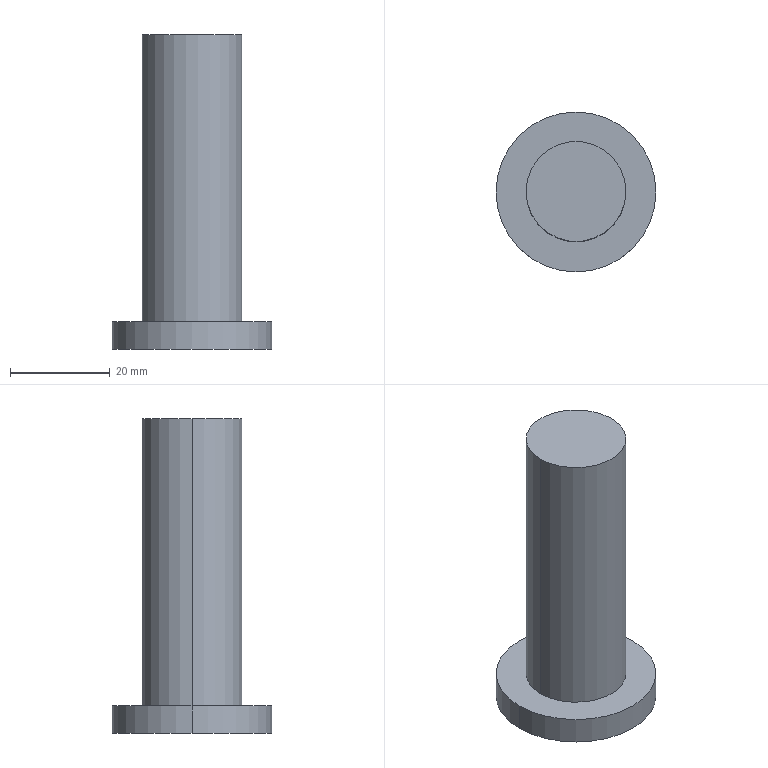Part | SolidWorks | features Extrusion 1, ICE 1 | 1 solid | 7 faces | box 32 x 32 x 63 mm | volume 22488 mm3 | cylinder 4 | plane 3 | commonest cylinder face diameters 20 x2 32 x2
STEP:
#1=CARTESIAN_POINT('',(16.,0.,5.5));
#2=VERTEX_POINT('',#1);
#3=CARTESIAN_POINT('',(-16.,0.,5.5));
#4=VERTEX_POINT('',#3);
#5=CARTESIAN_POINT('',(0.,0.,5.5));
#6=DIRECTION('',(0.,0.,1.));
#7=DIRECTION('',(1.,0.,0.));
#8=AXIS2_PLACEMENT_3D('',#5,#6,#7);
#9=CIRCLE('',#8,16.);
#10=EDGE_CURVE('',#2,#4,#9,.T.);
#11=ORIENTED_EDGE('',*,*,#10,.F.);
#12=CARTESIAN_POINT('',(16.,0.,0.));
#13=VERTEX_POINT('',#12);
#14=CARTESIAN_POINT('',(16.,0.,5.5));
#15=DIRECTION('',(0.,0.,-1.));
#16=VECTOR('',#15,1000.);
#17=LINE('',#14,#16);
#18=EDGE_CURVE('',#2,#13,#17,.T.);
#19=ORIENTED_EDGE('',*,*,#18,.T.);
#20=CARTESIAN_POINT('',(-16.,0.,0.));
#21=VERTEX_POINT('',#20);
#22=CARTESIAN_POINT('',(0.,0.,0.));
#23=DIRECTION('',(0.,0.,1.));
#24=DIRECTION('',(1.,0.,0.));
#25=AXIS2_PLACEMENT_3D('',#22,#23,#24);
#26=CIRCLE('',#25,16.);
#27=EDGE_CURVE('',#13,#21,#26,.T.);
#28=ORIENTED_EDGE('',*,*,#27,.T.);
#29=CARTESIAN_POINT('',(-16.,0.,5.5));
#30=DIRECTION('',(0.,0.,-1.));
#31=VECTOR('',#30,1000.);
#32=LINE('',#29,#31);
#33=EDGE_CURVE('',#4,#21,#32,.T.);
#34=ORIENTED_EDGE('',*,*,#33,.F.);
#35=EDGE_LOOP('',(#11,#19,#28,#34));
#36=FACE_OUTER_BOUND('',#35,.T.);
#37=CARTESIAN_POINT('',(0.,0.,5.5));
#38=DIRECTION('',(0.,0.,-1.));
#39=DIRECTION('',(-1.,0.,0.));
#40=AXIS2_PLACEMENT_3D('',#37,#38,#39);
#41=CYLINDRICAL_SURFACE('',#40,16.);
#42=ADVANCED_FACE('',(#36),#41,.T.);
#43=CARTESIAN_POINT('',(10.,0.,63.));
#44=VERTEX_POINT('',#43);
#45=CARTESIAN_POINT('',(-10.,0.,63.));
#46=VERTEX_POINT('',#45);
#47=CARTESIAN_POINT('',(0.,0.,63.));
#48=DIRECTION('',(0.,0.,1.));
#49=DIRECTION('',(1.,0.,0.));
#50=AXIS2_PLACEMENT_3D('',#47,#48,#49);
#51=CIRCLE('',#50,10.);
#52=EDGE_CURVE('',#44,#46,#51,.T.);
#53=ORIENTED_EDGE('',*,*,#52,.F.);
#54=CARTESIAN_POINT('',(10.,0.,5.5));
#55=VERTEX_POINT('',#54);
#56=CARTESIAN_POINT('',(10.,0.,63.));
#57=DIRECTION('',(0.,0.,-1.));
#58=VECTOR('',#57,1000.);
#59=LINE('',#56,#58);
#60=EDGE_CURVE('',#44,#55,#59,.T.);
#61=ORIENTED_EDGE('',*,*,#60,.T.);
#62=CARTESIAN_POINT('',(-10.,0.,5.5));
#63=VERTEX_POINT('',#62);
#64=CARTESIAN_POINT('',(0.,0.,5.5));
#65=DIRECTION('',(0.,0.,1.));
#66=DIRECTION('',(1.,0.,0.));
#67=AXIS2_PLACEMENT_3D('',#64,#65,#66);
#68=CIRCLE('',#67,10.);
#69=EDGE_CURVE('',#55,#63,#68,.T.);
#70=ORIENTED_EDGE('',*,*,#69,.T.);
#71=CARTESIAN_POINT('',(-10.,0.,63.));
#72=DIRECTION('',(0.,0.,-1.));
#73=VECTOR('',#72,1000.);
#74=LINE('',#71,#73);
#75=EDGE_CURVE('',#46,#63,#74,.T.);
#76=ORIENTED_EDGE('',*,*,#75,.F.);
#77=EDGE_LOOP('',(#53,#61,#70,#76));
#78=FACE_OUTER_BOUND('',#77,.T.);
#79=CARTESIAN_POINT('',(0.,0.,63.));
#80=DIRECTION('',(0.,0.,-1.));
#81=DIRECTION('',(-1.,0.,0.));
#82=AXIS2_PLACEMENT_3D('',#79,#80,#81);
#83=CYLINDRICAL_SURFACE('',#82,10.);
#84=ADVANCED_FACE('',(#78),#83,.T.);
#85=ORIENTED_EDGE('',*,*,#60,.F.);
#86=CARTESIAN_POINT('',(0.,0.,63.));
#87=DIRECTION('',(0.,0.,1.));
#88=DIRECTION('',(1.,0.,0.));
#89=AXIS2_PLACEMENT_3D('',#86,#87,#88);
#90=CIRCLE('',#89,10.);
#91=EDGE_CURVE('',#46,#44,#90,.T.);
#92=ORIENTED_EDGE('',*,*,#91,.F.);
#93=ORIENTED_EDGE('',*,*,#75,.T.);
#94=CARTESIAN_POINT('',(0.,0.,5.5));
#95=DIRECTION('',(0.,0.,1.));
#96=DIRECTION('',(1.,0.,0.));
#97=AXIS2_PLACEMENT_3D('',#94,#95,#96);
#98=CIRCLE('',#97,10.);
#99=EDGE_CURVE('',#63,#55,#98,.T.);
#100=ORIENTED_EDGE('',*,*,#99,.T.);
#101=EDGE_LOOP('',(#85,#92,#93,#100));
#102=FACE_OUTER_BOUND('',#101,.T.);
#103=CARTESIAN_POINT('',(0.,0.,63.));
#104=DIRECTION('',(0.,0.,-1.));
#105=DIRECTION('',(-1.,0.,0.));
#106=AXIS2_PLACEMENT_3D('',#103,#104,#105);
#107=CYLINDRICAL_SURFACE('',#106,10.);
#108=ADVANCED_FACE('',(#102),#107,.T.);
#109=ORIENTED_EDGE('',*,*,#91,.T.);
#110=ORIENTED_EDGE('',*,*,#52,.T.);
#111=EDGE_LOOP('',(#109,#110));
#112=FACE_OUTER_BOUND('',#111,.T.);
#113=CARTESIAN_POINT('',(0.,0.,63.));
#114=DIRECTION('',(0.,0.,1.));
#115=DIRECTION('',(1.,0.,0.));
#116=AXIS2_PLACEMENT_3D('',#113,#114,#115);
#117=PLANE('',#116);
#118=ADVANCED_FACE('',(#112),#117,.T.);
#119=ORIENTED_EDGE('',*,*,#18,.F.);
#120=CARTESIAN_POINT('',(0.,0.,5.5));
#121=DIRECTION('',(0.,0.,1.));
#122=DIRECTION('',(1.,0.,0.));
#123=AXIS2_PLACEMENT_3D('',#120,#121,#122);
#124=CIRCLE('',#123,16.);
#125=EDGE_CURVE('',#4,#2,#124,.T.);
#126=ORIENTED_EDGE('',*,*,#125,.F.);
#127=ORIENTED_EDGE('',*,*,#33,.T.);
#128=CARTESIAN_POINT('',(0.,0.,0.));
#129=DIRECTION('',(0.,0.,1.));
#130=DIRECTION('',(1.,0.,0.));
#131=AXIS2_PLACEMENT_3D('',#128,#129,#130);
#132=CIRCLE('',#131,16.);
#133=EDGE_CURVE('',#21,#13,#132,.T.);
#134=ORIENTED_EDGE('',*,*,#133,.T.);
#135=EDGE_LOOP('',(#119,#126,#127,#134));
#136=FACE_OUTER_BOUND('',#135,.T.);
#137=CARTESIAN_POINT('',(0.,0.,5.5));
#138=DIRECTION('',(0.,0.,-1.));
#139=DIRECTION('',(-1.,0.,0.));
#140=AXIS2_PLACEMENT_3D('',#137,#138,#139);
#141=CYLINDRICAL_SURFACE('',#140,16.);
#142=ADVANCED_FACE('',(#136),#141,.T.);
#143=ORIENTED_EDGE('',*,*,#99,.F.);
#144=ORIENTED_EDGE('',*,*,#69,.F.);
#145=EDGE_LOOP('',(#143,#144));
#146=FACE_BOUND('',#145,.T.);
#147=ORIENTED_EDGE('',*,*,#125,.T.);
#148=ORIENTED_EDGE('',*,*,#10,.T.);
#149=EDGE_LOOP('',(#147,#148));
#150=FACE_OUTER_BOUND('',#149,.T.);
#151=CARTESIAN_POINT('',(0.,0.,5.5));
#152=DIRECTION('',(0.,0.,1.));
#153=DIRECTION('',(1.,0.,0.));
#154=AXIS2_PLACEMENT_3D('',#151,#152,#153);
#155=PLANE('',#154);
#156=ADVANCED_FACE('',(#146,#150),#155,.T.);
#157=ORIENTED_EDGE('',*,*,#133,.F.);
#158=ORIENTED_EDGE('',*,*,#27,.F.);
#159=EDGE_LOOP('',(#157,#158));
#160=FACE_OUTER_BOUND('',#159,.T.);
#161=CARTESIAN_POINT('',(0.,0.,0.));
#162=DIRECTION('',(0.,0.,1.));
#163=DIRECTION('',(1.,0.,0.));
#164=AXIS2_PLACEMENT_3D('',#161,#162,#163);
#165=PLANE('',#164);
#166=ADVANCED_FACE('',(#160),#165,.F.);
#167=CLOSED_SHELL('',(#42,#84,#108,#118,#142,#156,#166));
#168=MANIFOLD_SOLID_BREP('',#167);
#169=CARTESIAN_POINT('',(0.,0.,0.));
#170=DIRECTION('',(0.,0.,1.));
#171=DIRECTION('',(1.,0.,0.));
#172=AXIS2_PLACEMENT_3D('',#169,#170,#171);
#173=(LENGTH_UNIT()NAMED_UNIT(*)SI_UNIT(.MILLI.,.METRE.));
#174=UNCERTAINTY_MEASURE_WITH_UNIT(LENGTH_MEASURE(0.00001),#173,'','');
#175=(NAMED_UNIT(*)PLANE_ANGLE_UNIT()SI_UNIT($,.RADIAN.));
#176=(NAMED_UNIT(*)SI_UNIT($,.STERADIAN.)SOLID_ANGLE_UNIT());
#177=(GEOMETRIC_REPRESENTATION_CONTEXT(3)GLOBAL_UNCERTAINTY_ASSIGNED_CONTEXT((#174))GLOBAL_UNIT_ASSIGNED_CONTEXT((#173,#175,#176))REPRESENTATION_CONTEXT('',''));
#178=ADVANCED_BREP_SHAPE_REPRESENTATION('',(#168,#172),#177);